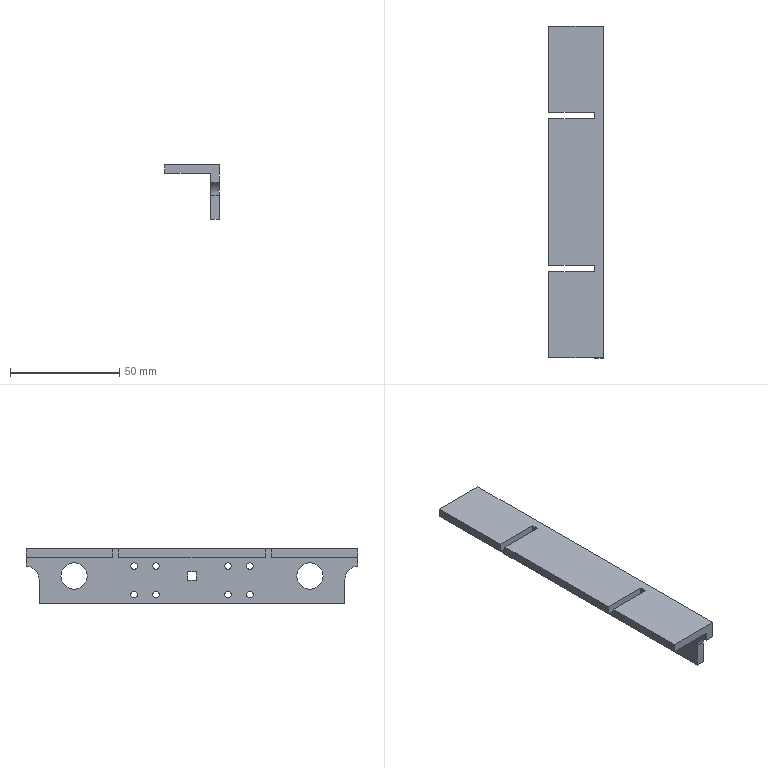Part | STEP file | 1-01.2 | 1 solid | 34 faces | box 25 x 152 x 25 mm | volume 25515 mm3 | plane 22 | cylinder 12 | commonest cylinder face diameters 3 x8 12 x4